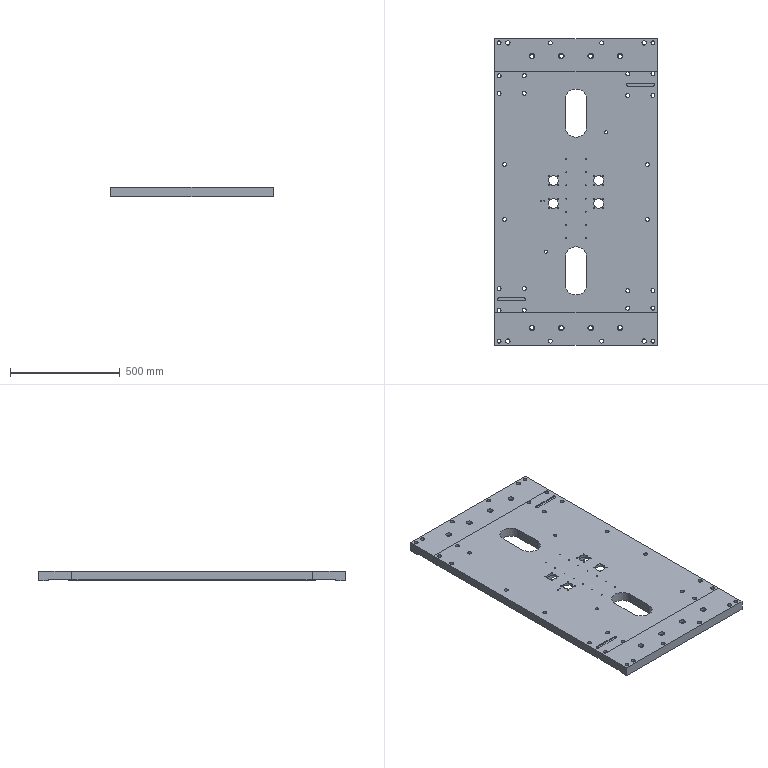Part | STEP file | LM-05-1222B_default | 1 solid | 525 faces | box 742 x 1400 x 44 mm | volume 38795676 mm3 | cylinder 334 | plane 98 | cone 82 | spline 11 | commonest cylinder face diameters 26 x72 6.8 x60 5 x58 18 x56 4.2 x28 19 x16